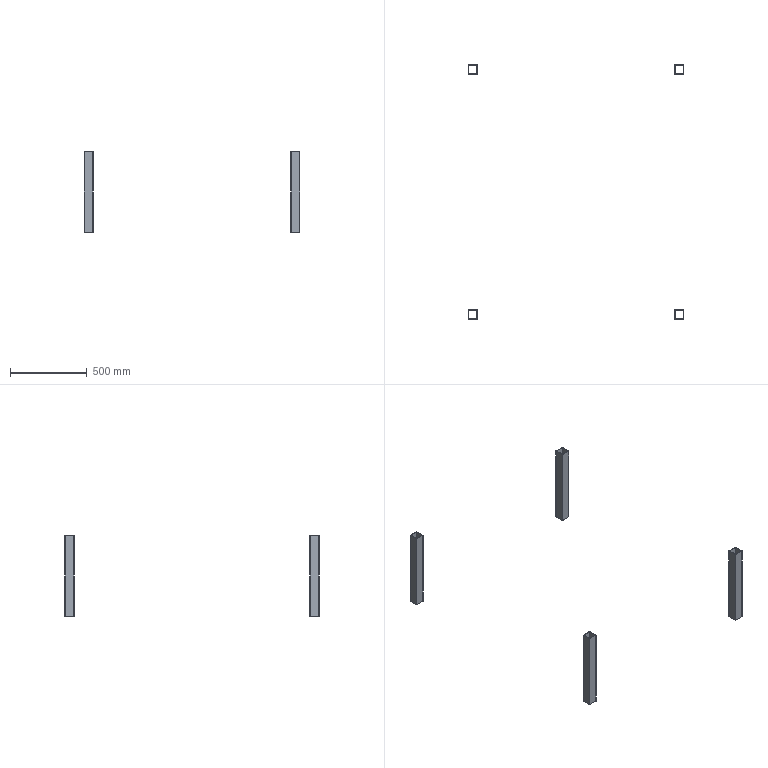Part | STEP file | ASND-0110-E63-HLTP01 square steel frame | 4 solids | 40 faces | box 1400 x 1650 x 525 mm | volume 1881600 mm3 | plane 40